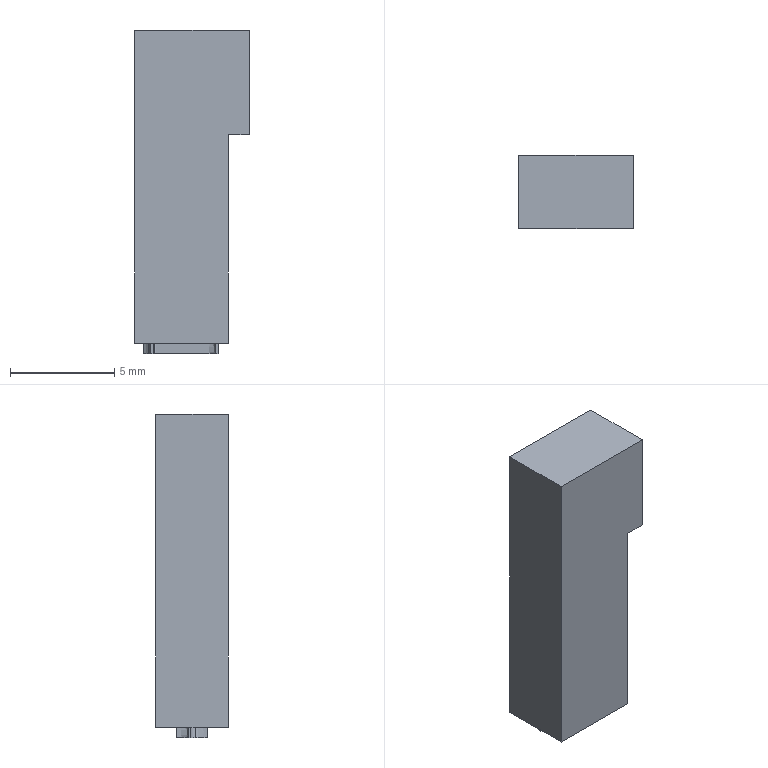Part | STEP file | gslz 2016.10.28-10_id1654_x_t | 1 solid | 19 faces | box 5.5 x 3.5 x 15.5 mm | volume 254.454 mm3 | plane 14 | other 5